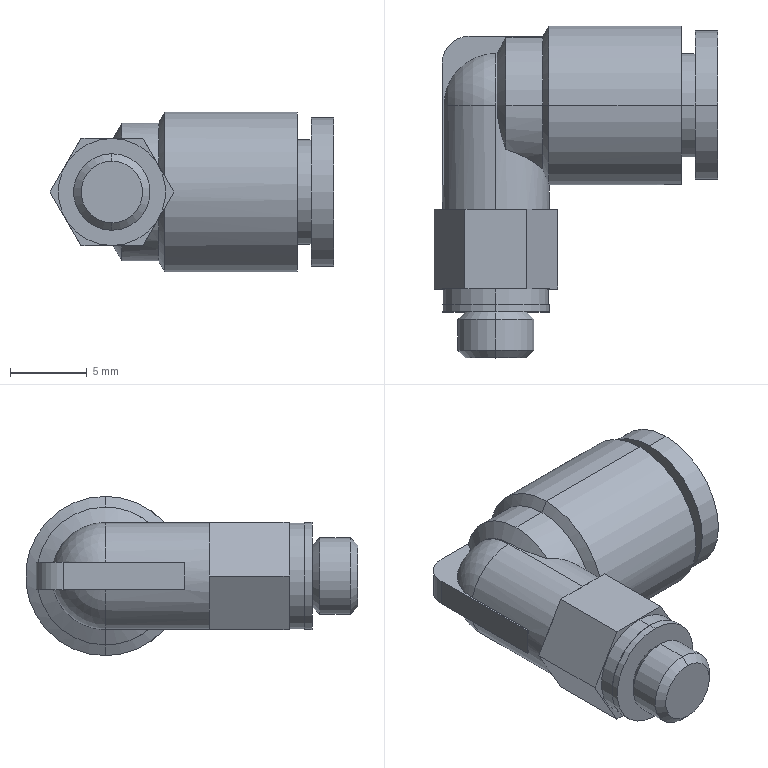Part | NX | features BREP 1 | 1 solid | 61 faces | box 18.541 x 21.7 x 10.4 mm | volume 1291 mm3 | plane 26 | cylinder 23 | cone 10 | sphere 2 | commonest cylinder face diameters 7 x7 9 x3 5 x2 6 x2 6.8 x2 6.9 x2